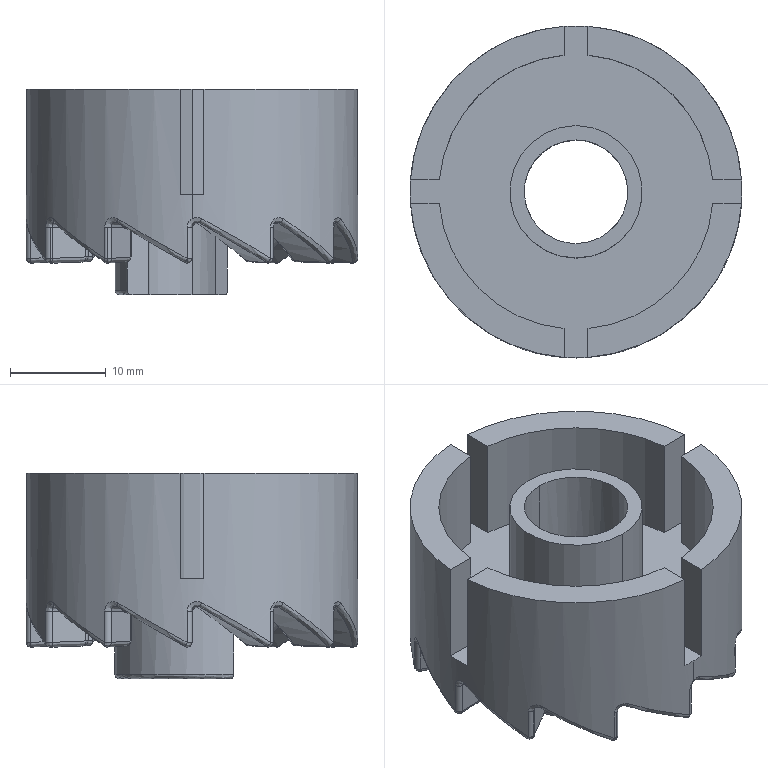Part | SolidWorks | features BaseBody 1 | 1 solid | 200 faces | box 34.702 x 34.702 x 21.496 mm | volume 7311 mm3 | spline 127 | cylinder 43 | plane 30 | commonest cylinder face diameters 1.003 x29 28.684 x4 10.832 x2 13.841 x2 16.126 x2 24.672 x2